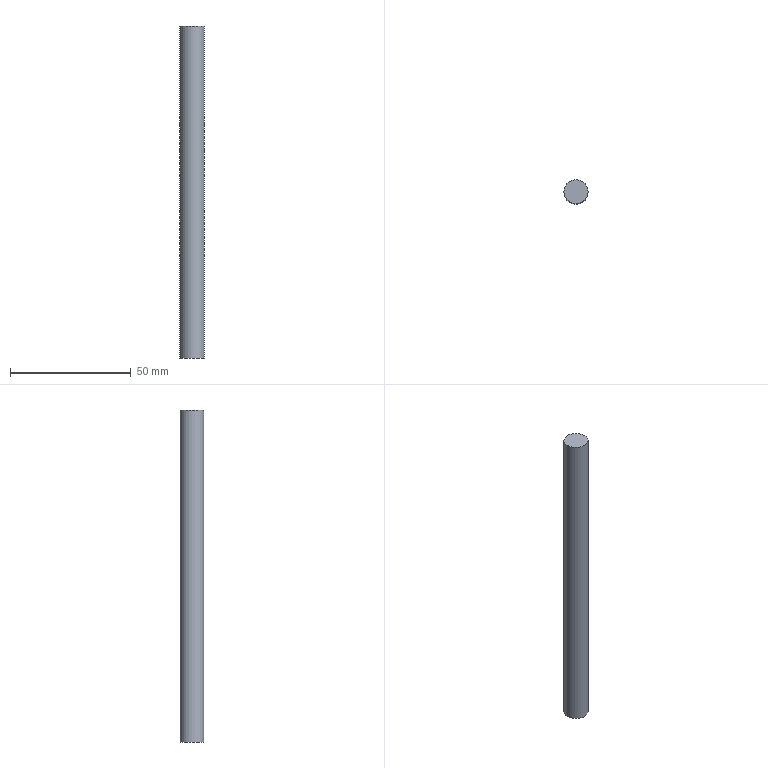Part | STEP file | solid 104 | 1 solid | 3 faces | box 10 x 10 x 137.677 mm | volume 10813 mm3 | plane 2 | cylinder 1 | commonest cylinder face diameters 10 x1